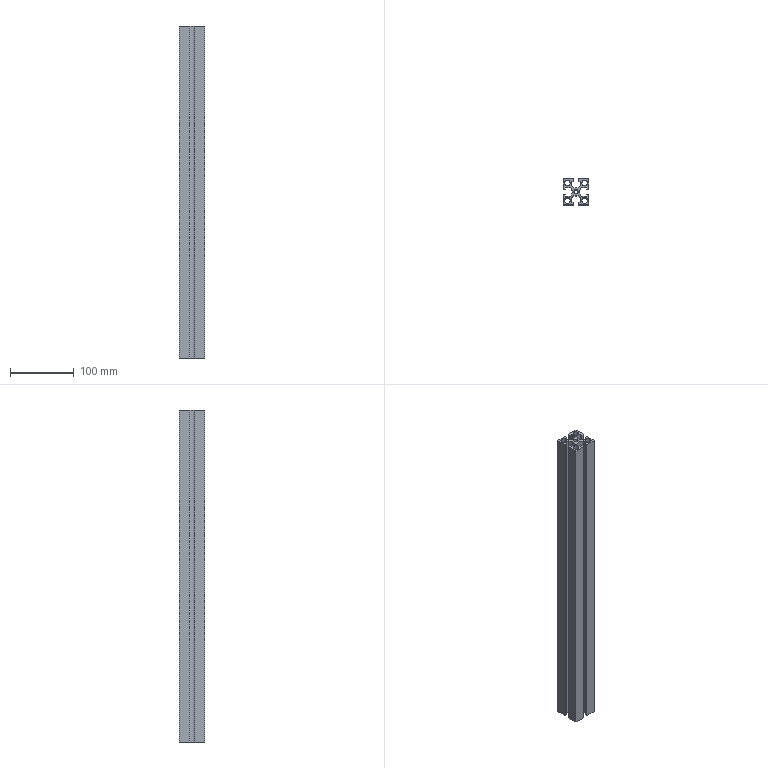Part | STEP file | Frame aluminum channel 3 | 1 solid | 49 faces | box 40 x 40 x 520 mm | volume 336590 mm3 | plane 34 | cylinder 15 | commonest cylinder face diameters 9 x8 19.803 x5 7 x2